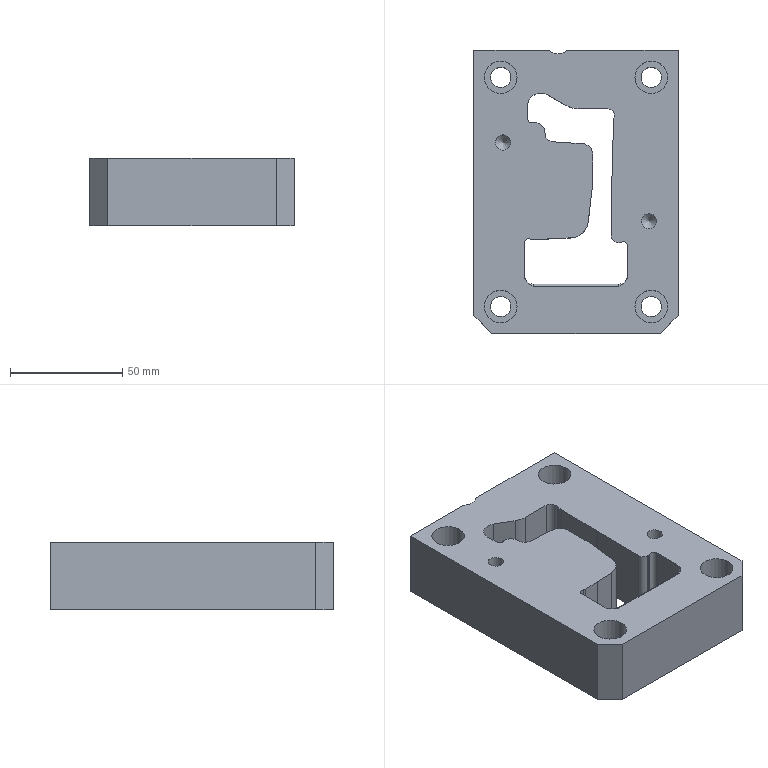Part | NX | features solid 2 | 1 solid | 71 faces | box 91 x 126 x 30 mm | volume 269999 mm3 | plane 41 | cylinder 26 | cone 2 | torus 2 | commonest cylinder face diameters 4 x6 9 x4 14.5 x4 6 x3 6.8 x2 8 x2